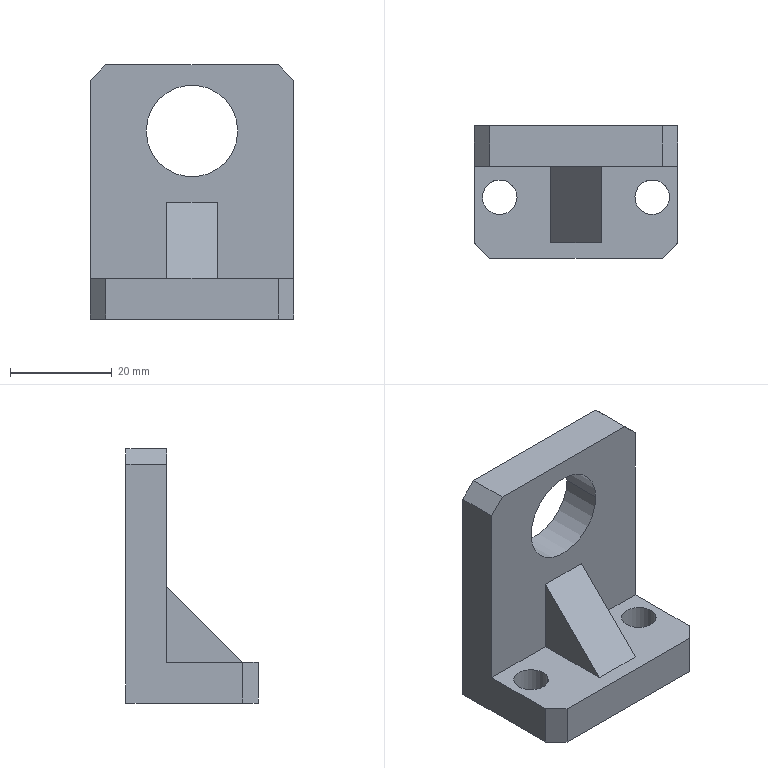Part | STEP file | 20315 | 1 solid | 21 faces | box 40 x 26 x 50 mm | volume 20124 mm3 | plane 15 | cylinder 6 | commonest cylinder face diameters 6.8 x4 18 x2
STEP:
#1=CARTESIAN_POINT('',(-17.984,13.63,0.));
#2=VERTEX_POINT('',#1);
#3=CARTESIAN_POINT('',(-17.984,13.63,8.));
#4=VERTEX_POINT('',#3);
#5=CARTESIAN_POINT('',(-17.984,13.63,24.155));
#6=DIRECTION('',(0.,0.,-1.));
#7=VECTOR('',#6,1.);
#8=LINE('',#5,#7);
#9=EDGE_CURVE('',#2,#4,#8,.F.);
#10=ORIENTED_EDGE('',*,*,#9,.F.);
#11=CARTESIAN_POINT('',(-12.016,10.37,0.));
#12=VERTEX_POINT('',#11);
#13=CARTESIAN_POINT('',(-15.,12.,0.));
#14=DIRECTION('',(0.,0.,-1.));
#15=AXIS2_PLACEMENT_3D('',#13,#14,$);
#16=CIRCLE('',#15,3.4);
#17=EDGE_CURVE('',#2,#12,#16,.T.);
#18=ORIENTED_EDGE('',*,*,#17,.T.);
#19=CARTESIAN_POINT('',(-12.016,10.37,8.));
#20=VERTEX_POINT('',#19);
#21=CARTESIAN_POINT('',(-12.016,10.37,24.155));
#22=DIRECTION('',(0.,0.,-1.));
#23=VECTOR('',#22,1.);
#24=LINE('',#21,#23);
#25=EDGE_CURVE('',#12,#20,#24,.F.);
#26=ORIENTED_EDGE('',*,*,#25,.T.);
#27=CARTESIAN_POINT('',(-15.,12.,8.));
#28=DIRECTION('',(0.,0.,-1.));
#29=AXIS2_PLACEMENT_3D('',#27,#28,$);
#30=CIRCLE('',#29,3.4);
#31=EDGE_CURVE('',#20,#4,#30,.F.);
#32=ORIENTED_EDGE('',*,*,#31,.T.);
#33=EDGE_LOOP('',(#10,#18,#26,#32));
#34=FACE_OUTER_BOUND('',#33,.T.);
#35=CARTESIAN_POINT('',(-15.,12.,7.9));
#36=DIRECTION('',(0.,0.,-1.));
#37=DIRECTION('',(0.8776,-0.4794,0.));
#38=AXIS2_PLACEMENT_3D('',#35,#36,#37);
#39=CYLINDRICAL_SURFACE('',#38,3.4);
#40=ADVANCED_FACE('',(#34),#39,.F.);
#41=ORIENTED_EDGE('',*,*,#25,.F.);
#42=CARTESIAN_POINT('',(-15.,12.,0.));
#43=DIRECTION('',(0.,0.,-1.));
#44=AXIS2_PLACEMENT_3D('',#42,#43,$);
#45=CIRCLE('',#44,3.4);
#46=EDGE_CURVE('',#12,#2,#45,.T.);
#47=ORIENTED_EDGE('',*,*,#46,.T.);
#48=ORIENTED_EDGE('',*,*,#9,.T.);
#49=CARTESIAN_POINT('',(-15.,12.,8.));
#50=DIRECTION('',(0.,0.,-1.));
#51=AXIS2_PLACEMENT_3D('',#49,#50,$);
#52=CIRCLE('',#51,3.4);
#53=EDGE_CURVE('',#4,#20,#52,.F.);
#54=ORIENTED_EDGE('',*,*,#53,.T.);
#55=EDGE_LOOP('',(#41,#47,#48,#54));
#56=FACE_OUTER_BOUND('',#55,.T.);
#57=ADVANCED_FACE('',(#56),#39,.F.);
#58=CARTESIAN_POINT('',(-5.,18.,8.));
#59=VERTEX_POINT('',#58);
#60=CARTESIAN_POINT('',(-5.,18.,23.));
#61=VERTEX_POINT('',#60);
#62=CARTESIAN_POINT('',(-5.,18.,15.5));
#63=DIRECTION('',(0.,0.,1.));
#64=VECTOR('',#63,1.);
#65=LINE('',#62,#64);
#66=EDGE_CURVE('',#59,#61,#65,.T.);
#67=ORIENTED_EDGE('',*,*,#66,.F.);
#68=CARTESIAN_POINT('',(-5.,3.,8.));
#69=VERTEX_POINT('',#68);
#70=CARTESIAN_POINT('',(-5.,10.5,8.));
#71=DIRECTION('',(0.,1.,0.));
#72=VECTOR('',#71,1.);
#73=LINE('',#70,#72);
#74=EDGE_CURVE('',#69,#59,#73,.T.);
#75=ORIENTED_EDGE('',*,*,#74,.F.);
#76=CARTESIAN_POINT('',(-5.,10.5,15.5));
#77=DIRECTION('',(0.,-0.7071,-0.7071));
#78=VECTOR('',#77,1.);
#79=LINE('',#76,#78);
#80=EDGE_CURVE('',#61,#69,#79,.T.);
#81=ORIENTED_EDGE('',*,*,#80,.F.);
#82=EDGE_LOOP('',(#67,#75,#81));
#83=FACE_OUTER_BOUND('',#82,.T.);
#84=CARTESIAN_POINT('',(-5.,0.,0.));
#85=DIRECTION('',(1.,0.,0.));
#86=DIRECTION('',(0.,1.,0.));
#87=AXIS2_PLACEMENT_3D('',#84,#85,#86);
#88=PLANE('',#87);
#89=ADVANCED_FACE('',(#83),#88,.F.);
#90=CARTESIAN_POINT('',(-20.,3.,8.));
#91=VERTEX_POINT('',#90);
#92=CARTESIAN_POINT('',(-20.,3.,0.));
#93=VERTEX_POINT('',#92);
#94=CARTESIAN_POINT('',(-20.,3.,4.));
#95=DIRECTION('',(0.,0.,-1.));
#96=VECTOR('',#95,1.);
#97=LINE('',#94,#96);
#98=EDGE_CURVE('',#91,#93,#97,.T.);
#99=ORIENTED_EDGE('',*,*,#98,.F.);
#100=CARTESIAN_POINT('',(-20.,18.,8.));
#101=VERTEX_POINT('',#100);
#102=CARTESIAN_POINT('',(-20.,10.5,8.));
#103=DIRECTION('',(0.,-1.,0.));
#104=VECTOR('',#103,1.);
#105=LINE('',#102,#104);
#106=EDGE_CURVE('',#101,#91,#105,.T.);
#107=ORIENTED_EDGE('',*,*,#106,.F.);
#108=CARTESIAN_POINT('',(-20.,18.,47.));
#109=VERTEX_POINT('',#108);
#110=CARTESIAN_POINT('',(-20.,18.,27.5));
#111=DIRECTION('',(0.,0.,-1.));
#112=VECTOR('',#111,1.);
#113=LINE('',#110,#112);
#114=EDGE_CURVE('',#109,#101,#113,.T.);
#115=ORIENTED_EDGE('',*,*,#114,.F.);
#116=CARTESIAN_POINT('',(-20.,26.,47.));
#117=VERTEX_POINT('',#116);
#118=CARTESIAN_POINT('',(-20.,22.,47.));
#119=DIRECTION('',(0.,1.,0.));
#120=VECTOR('',#119,1.);
#121=LINE('',#118,#120);
#122=EDGE_CURVE('',#117,#109,#121,.F.);
#123=ORIENTED_EDGE('',*,*,#122,.F.);
#124=CARTESIAN_POINT('',(-20.,26.,0.));
#125=VERTEX_POINT('',#124);
#126=CARTESIAN_POINT('',(-20.,26.,23.5));
#127=DIRECTION('',(0.,0.,1.));
#128=VECTOR('',#127,1.);
#129=LINE('',#126,#128);
#130=EDGE_CURVE('',#125,#117,#129,.T.);
#131=ORIENTED_EDGE('',*,*,#130,.F.);
#132=CARTESIAN_POINT('',(-20.,14.5,0.));
#133=DIRECTION('',(0.,1.,0.));
#134=VECTOR('',#133,1.);
#135=LINE('',#132,#134);
#136=EDGE_CURVE('',#93,#125,#135,.T.);
#137=ORIENTED_EDGE('',*,*,#136,.F.);
#138=EDGE_LOOP('',(#99,#107,#115,#123,#131,#137));
#139=FACE_OUTER_BOUND('',#138,.T.);
#140=CARTESIAN_POINT('',(-20.,0.,0.));
#141=DIRECTION('',(1.,0.,0.));
#142=DIRECTION('',(0.,1.,0.));
#143=AXIS2_PLACEMENT_3D('',#140,#141,#142);
#144=PLANE('',#143);
#145=ADVANCED_FACE('',(#139),#144,.F.);
#146=CARTESIAN_POINT('',(-17.,0.,8.));
#147=VERTEX_POINT('',#146);
#148=CARTESIAN_POINT('',(17.,0.,8.));
#149=VERTEX_POINT('',#148);
#150=CARTESIAN_POINT('',(0.,0.,8.));
#151=DIRECTION('',(1.,0.,0.));
#152=VECTOR('',#151,1.);
#153=LINE('',#150,#152);
#154=EDGE_CURVE('',#147,#149,#153,.T.);
#155=ORIENTED_EDGE('',*,*,#154,.F.);
#156=CARTESIAN_POINT('',(-17.,0.,0.));
#157=VERTEX_POINT('',#156);
#158=CARTESIAN_POINT('',(-17.,0.,4.));
#159=DIRECTION('',(0.,0.,-1.));
#160=VECTOR('',#159,1.);
#161=LINE('',#158,#160);
#162=EDGE_CURVE('',#147,#157,#161,.T.);
#163=ORIENTED_EDGE('',*,*,#162,.T.);
#164=CARTESIAN_POINT('',(17.,0.,0.));
#165=VERTEX_POINT('',#164);
#166=CARTESIAN_POINT('',(0.,0.,0.));
#167=DIRECTION('',(1.,0.,0.));
#168=VECTOR('',#167,1.);
#169=LINE('',#166,#168);
#170=EDGE_CURVE('',#157,#165,#169,.T.);
#171=ORIENTED_EDGE('',*,*,#170,.T.);
#172=CARTESIAN_POINT('',(17.,0.,4.));
#173=DIRECTION('',(0.,0.,-1.));
#174=VECTOR('',#173,1.);
#175=LINE('',#172,#174);
#176=EDGE_CURVE('',#149,#165,#175,.T.);
#177=ORIENTED_EDGE('',*,*,#176,.F.);
#178=EDGE_LOOP('',(#155,#163,#171,#177));
#179=FACE_OUTER_BOUND('',#178,.T.);
#180=CARTESIAN_POINT('',(0.,0.,8.));
#181=DIRECTION('',(0.,-1.,0.));
#182=DIRECTION('',(0.,0.,-1.));
#183=AXIS2_PLACEMENT_3D('',#180,#181,#182);
#184=PLANE('',#183);
#185=ADVANCED_FACE('',(#179),#184,.T.);
#186=CARTESIAN_POINT('',(-17.,18.,50.));
#187=VERTEX_POINT('',#186);
#188=CARTESIAN_POINT('',(17.,18.,50.));
#189=VERTEX_POINT('',#188);
#190=CARTESIAN_POINT('',(0.,18.,50.));
#191=DIRECTION('',(1.,0.,0.));
#192=VECTOR('',#191,1.);
#193=LINE('',#190,#192);
#194=EDGE_CURVE('',#187,#189,#193,.T.);
#195=ORIENTED_EDGE('',*,*,#194,.T.);
#196=CARTESIAN_POINT('',(17.,26.,50.));
#197=VERTEX_POINT('',#196);
#198=CARTESIAN_POINT('',(17.,22.,50.));
#199=DIRECTION('',(0.,1.,0.));
#200=VECTOR('',#199,1.);
#201=LINE('',#198,#200);
#202=EDGE_CURVE('',#197,#189,#201,.F.);
#203=ORIENTED_EDGE('',*,*,#202,.F.);
#204=CARTESIAN_POINT('',(-17.,26.,50.));
#205=VERTEX_POINT('',#204);
#206=CARTESIAN_POINT('',(0.,26.,50.));
#207=DIRECTION('',(1.,0.,0.));
#208=VECTOR('',#207,1.);
#209=LINE('',#206,#208);
#210=EDGE_CURVE('',#205,#197,#209,.T.);
#211=ORIENTED_EDGE('',*,*,#210,.F.);
#212=CARTESIAN_POINT('',(-17.,22.,50.));
#213=DIRECTION('',(0.,1.,0.));
#214=VECTOR('',#213,1.);
#215=LINE('',#212,#214);
#216=EDGE_CURVE('',#205,#187,#215,.F.);
#217=ORIENTED_EDGE('',*,*,#216,.T.);
#218=EDGE_LOOP('',(#195,#203,#211,#217));
#219=FACE_OUTER_BOUND('',#218,.T.);
#220=CARTESIAN_POINT('',(0.,26.,50.));
#221=DIRECTION('',(0.,0.,1.));
#222=DIRECTION('',(0.,-1.,0.));
#223=AXIS2_PLACEMENT_3D('',#220,#221,#222);
#224=PLANE('',#223);
#225=ADVANCED_FACE('',(#219),#224,.T.);
#226=CARTESIAN_POINT('',(20.,26.,47.));
#227=VERTEX_POINT('',#226);
#228=CARTESIAN_POINT('',(20.,18.,47.));
#229=VERTEX_POINT('',#228);
#230=CARTESIAN_POINT('',(20.,13.,47.));
#231=DIRECTION('',(0.,1.,0.));
#232=VECTOR('',#231,1.);
#233=LINE('',#230,#232);
#234=EDGE_CURVE('',#227,#229,#233,.F.);
#235=ORIENTED_EDGE('',*,*,#234,.F.);
#236=CARTESIAN_POINT('',(18.5,26.,48.5));
#237=DIRECTION('',(0.7071,0.,-0.7071));
#238=VECTOR('',#237,1.);
#239=LINE('',#236,#238);
#240=EDGE_CURVE('',#227,#197,#239,.F.);
#241=ORIENTED_EDGE('',*,*,#240,.T.);
#242=ORIENTED_EDGE('',*,*,#202,.T.);
#243=CARTESIAN_POINT('',(18.5,18.,48.5));
#244=DIRECTION('',(0.7071,0.,-0.7071));
#245=VECTOR('',#244,1.);
#246=LINE('',#243,#245);
#247=EDGE_CURVE('',#189,#229,#246,.T.);
#248=ORIENTED_EDGE('',*,*,#247,.T.);
#249=EDGE_LOOP('',(#235,#241,#242,#248));
#250=FACE_OUTER_BOUND('',#249,.T.);
#251=CARTESIAN_POINT('',(17.,-5.2,50.));
#252=DIRECTION('',(-0.7071,0.,-0.7071));
#253=DIRECTION('',(0.,1.,0.));
#254=AXIS2_PLACEMENT_3D('',#251,#252,#253);
#255=PLANE('',#254);
#256=ADVANCED_FACE('',(#250),#255,.F.);
#257=CARTESIAN_POINT('',(-18.5,18.,48.5));
#258=DIRECTION('',(-0.7071,0.,-0.7071));
#259=VECTOR('',#258,1.);
#260=LINE('',#257,#259);
#261=EDGE_CURVE('',#109,#187,#260,.F.);
#262=ORIENTED_EDGE('',*,*,#261,.T.);
#263=ORIENTED_EDGE('',*,*,#216,.F.);
#264=CARTESIAN_POINT('',(-18.5,26.,48.5));
#265=DIRECTION('',(-0.7071,0.,-0.7071));
#266=VECTOR('',#265,1.);
#267=LINE('',#264,#266);
#268=EDGE_CURVE('',#205,#117,#267,.T.);
#269=ORIENTED_EDGE('',*,*,#268,.T.);
#270=ORIENTED_EDGE('',*,*,#122,.T.);
#271=EDGE_LOOP('',(#262,#263,#269,#270));
#272=FACE_OUTER_BOUND('',#271,.T.);
#273=CARTESIAN_POINT('',(-17.,-5.2,50.));
#274=DIRECTION('',(-0.7071,0.,0.7071));
#275=DIRECTION('',(0.,1.,0.));
#276=AXIS2_PLACEMENT_3D('',#273,#274,#275);
#277=PLANE('',#276);
#278=ADVANCED_FACE('',(#272),#277,.T.);
#279=CARTESIAN_POINT('',(20.,3.,8.));
#280=VERTEX_POINT('',#279);
#281=CARTESIAN_POINT('',(20.,3.,0.));
#282=VERTEX_POINT('',#281);
#283=CARTESIAN_POINT('',(20.,3.,23.5));
#284=DIRECTION('',(0.,0.,-1.));
#285=VECTOR('',#284,1.);
#286=LINE('',#283,#285);
#287=EDGE_CURVE('',#280,#282,#286,.T.);
#288=ORIENTED_EDGE('',*,*,#287,.F.);
#289=CARTESIAN_POINT('',(18.5,1.5,8.));
#290=DIRECTION('',(-0.7071,-0.7071,0.));
#291=VECTOR('',#290,1.);
#292=LINE('',#289,#291);
#293=EDGE_CURVE('',#280,#149,#292,.T.);
#294=ORIENTED_EDGE('',*,*,#293,.T.);
#295=ORIENTED_EDGE('',*,*,#176,.T.);
#296=CARTESIAN_POINT('',(18.5,1.5,0.));
#297=DIRECTION('',(-0.7071,-0.7071,0.));
#298=VECTOR('',#297,1.);
#299=LINE('',#296,#298);
#300=EDGE_CURVE('',#165,#282,#299,.F.);
#301=ORIENTED_EDGE('',*,*,#300,.T.);
#302=EDGE_LOOP('',(#288,#294,#295,#301));
#303=FACE_OUTER_BOUND('',#302,.T.);
#304=CARTESIAN_POINT('',(20.,3.,56.4));
#305=DIRECTION('',(-0.7071,0.7071,0.));
#306=DIRECTION('',(0.,0.,-1.));
#307=AXIS2_PLACEMENT_3D('',#304,#305,#306);
#308=PLANE('',#307);
#309=ADVANCED_FACE('',(#303),#308,.F.);
#310=CARTESIAN_POINT('',(-18.5,1.5,0.));
#311=DIRECTION('',(0.7071,-0.7071,0.));
#312=VECTOR('',#311,1.);
#313=LINE('',#310,#312);
#314=EDGE_CURVE('',#93,#157,#313,.T.);
#315=ORIENTED_EDGE('',*,*,#314,.T.);
#316=ORIENTED_EDGE('',*,*,#162,.F.);
#317=CARTESIAN_POINT('',(-18.5,1.5,8.));
#318=DIRECTION('',(0.7071,-0.7071,0.));
#319=VECTOR('',#318,1.);
#320=LINE('',#317,#319);
#321=EDGE_CURVE('',#147,#91,#320,.F.);
#322=ORIENTED_EDGE('',*,*,#321,.T.);
#323=ORIENTED_EDGE('',*,*,#98,.T.);
#324=EDGE_LOOP('',(#315,#316,#322,#323));
#325=FACE_OUTER_BOUND('',#324,.T.);
#326=CARTESIAN_POINT('',(-20.,3.,56.4));
#327=DIRECTION('',(-0.7071,-0.7071,0.));
#328=DIRECTION('',(0.,0.,-1.));
#329=AXIS2_PLACEMENT_3D('',#326,#327,#328);
#330=PLANE('',#329);
#331=ADVANCED_FACE('',(#325),#330,.T.);
#332=CARTESIAN_POINT('',(5.,18.,23.));
#333=VERTEX_POINT('',#332);
#334=CARTESIAN_POINT('',(0.,18.,23.));
#335=DIRECTION('',(1.,0.,0.));
#336=VECTOR('',#335,1.);
#337=LINE('',#334,#336);
#338=EDGE_CURVE('',#61,#333,#337,.T.);
#339=ORIENTED_EDGE('',*,*,#338,.F.);
#340=ORIENTED_EDGE('',*,*,#80,.T.);
#341=CARTESIAN_POINT('',(5.,3.,8.));
#342=VERTEX_POINT('',#341);
#343=CARTESIAN_POINT('',(0.,3.,8.));
#344=DIRECTION('',(1.,0.,0.));
#345=VECTOR('',#344,1.);
#346=LINE('',#343,#345);
#347=EDGE_CURVE('',#69,#342,#346,.T.);
#348=ORIENTED_EDGE('',*,*,#347,.T.);
#349=CARTESIAN_POINT('',(5.,10.5,15.5));
#350=DIRECTION('',(0.,-0.7071,-0.7071));
#351=VECTOR('',#350,1.);
#352=LINE('',#349,#351);
#353=EDGE_CURVE('',#333,#342,#352,.T.);
#354=ORIENTED_EDGE('',*,*,#353,.F.);
#355=EDGE_LOOP('',(#339,#340,#348,#354));
#356=FACE_OUTER_BOUND('',#355,.T.);
#357=CARTESIAN_POINT('',(0.,18.,23.));
#358=DIRECTION('',(0.,-0.7071,0.7071));
#359=DIRECTION('',(0.,-0.7071,-0.7071));
#360=AXIS2_PLACEMENT_3D('',#357,#358,#359);
#361=PLANE('',#360);
#362=ADVANCED_FACE('',(#356),#361,.T.);
#363=ORIENTED_EDGE('',*,*,#353,.T.);
#364=CARTESIAN_POINT('',(5.,18.,8.));
#365=VERTEX_POINT('',#364);
#366=CARTESIAN_POINT('',(5.,10.5,8.));
#367=DIRECTION('',(0.,1.,0.));
#368=VECTOR('',#367,1.);
#369=LINE('',#366,#368);
#370=EDGE_CURVE('',#342,#365,#369,.T.);
#371=ORIENTED_EDGE('',*,*,#370,.T.);
#372=CARTESIAN_POINT('',(5.,18.,15.5));
#373=DIRECTION('',(0.,0.,1.));
#374=VECTOR('',#373,1.);
#375=LINE('',#372,#374);
#376=EDGE_CURVE('',#365,#333,#375,.T.);
#377=ORIENTED_EDGE('',*,*,#376,.T.);
#378=EDGE_LOOP('',(#363,#371,#377));
#379=FACE_OUTER_BOUND('',#378,.T.);
#380=CARTESIAN_POINT('',(5.,0.,0.));
#381=DIRECTION('',(1.,0.,0.));
#382=DIRECTION('',(0.,1.,0.));
#383=AXIS2_PLACEMENT_3D('',#380,#381,#382);
#384=PLANE('',#383);
#385=ADVANCED_FACE('',(#379),#384,.T.);
#386=CARTESIAN_POINT('',(20.,26.,0.));
#387=VERTEX_POINT('',#386);
#388=CARTESIAN_POINT('',(20.,14.5,0.));
#389=DIRECTION('',(0.,1.,0.));
#390=VECTOR('',#389,1.);
#391=LINE('',#388,#390);
#392=EDGE_CURVE('',#282,#387,#391,.T.);
#393=ORIENTED_EDGE('',*,*,#392,.T.);
#394=CARTESIAN_POINT('',(20.,26.,23.5));
#395=DIRECTION('',(0.,0.,1.));
#396=VECTOR('',#395,1.);
#397=LINE('',#394,#396);
#398=EDGE_CURVE('',#387,#227,#397,.T.);
#399=ORIENTED_EDGE('',*,*,#398,.T.);
#400=ORIENTED_EDGE('',*,*,#234,.T.);
#401=CARTESIAN_POINT('',(20.,18.,8.));
#402=VERTEX_POINT('',#401);
#403=CARTESIAN_POINT('',(20.,18.,27.5));
#404=DIRECTION('',(0.,0.,-1.));
#405=VECTOR('',#404,1.);
#406=LINE('',#403,#405);
#407=EDGE_CURVE('',#229,#402,#406,.T.);
#408=ORIENTED_EDGE('',*,*,#407,.T.);
#409=CARTESIAN_POINT('',(20.,10.5,8.));
#410=DIRECTION('',(0.,-1.,0.));
#411=VECTOR('',#410,1.);
#412=LINE('',#409,#411);
#413=EDGE_CURVE('',#402,#280,#412,.T.);
#414=ORIENTED_EDGE('',*,*,#413,.T.);
#415=ORIENTED_EDGE('',*,*,#287,.T.);
#416=EDGE_LOOP('',(#393,#399,#400,#408,#414,#415));
#417=FACE_OUTER_BOUND('',#416,.T.);
#418=CARTESIAN_POINT('',(20.,0.,0.));
#419=DIRECTION('',(1.,0.,0.));
#420=DIRECTION('',(0.,1.,0.));
#421=AXIS2_PLACEMENT_3D('',#418,#419,#420);
#422=PLANE('',#421);
#423=ADVANCED_FACE('',(#417),#422,.T.);
#424=ORIENTED_EDGE('',*,*,#170,.F.);
#425=ORIENTED_EDGE('',*,*,#314,.F.);
#426=ORIENTED_EDGE('',*,*,#136,.T.);
#427=CARTESIAN_POINT('',(0.,26.,0.));
#428=DIRECTION('',(1.,0.,0.));
#429=VECTOR('',#428,1.);
#430=LINE('',#427,#429);
#431=EDGE_CURVE('',#125,#387,#430,.T.);
#432=ORIENTED_EDGE('',*,*,#431,.T.);
#433=ORIENTED_EDGE('',*,*,#392,.F.);
#434=ORIENTED_EDGE('',*,*,#300,.F.);
#435=EDGE_LOOP('',(#424,#425,#426,#432,#433,#434));
#436=FACE_OUTER_BOUND('',#435,.T.);
#437=CARTESIAN_POINT('',(12.016,13.63,0.));
#438=VERTEX_POINT('',#437);
#439=CARTESIAN_POINT('',(17.984,10.37,0.));
#440=VERTEX_POINT('',#439);
#441=CARTESIAN_POINT('',(15.,12.,0.));
#442=DIRECTION('',(0.,0.,-1.));
#443=AXIS2_PLACEMENT_3D('',#441,#442,$);
#444=CIRCLE('',#443,3.4);
#445=EDGE_CURVE('',#438,#440,#444,.T.);
#446=ORIENTED_EDGE('',*,*,#445,.F.);
#447=CARTESIAN_POINT('',(15.,12.,0.));
#448=DIRECTION('',(0.,0.,-1.));
#449=AXIS2_PLACEMENT_3D('',#447,#448,$);
#450=CIRCLE('',#449,3.4);
#451=EDGE_CURVE('',#440,#438,#450,.T.);
#452=ORIENTED_EDGE('',*,*,#451,.F.);
#453=EDGE_LOOP('',(#446,#452));
#454=FACE_BOUND('',#453,.T.);
#455=ORIENTED_EDGE('',*,*,#46,.F.);
#456=ORIENTED_EDGE('',*,*,#17,.F.);
#457=EDGE_LOOP('',(#455,#456));
#458=FACE_BOUND('',#457,.T.);
#459=CARTESIAN_POINT('',(0.,0.,0.));
#460=DIRECTION('',(0.,0.,-1.));
#461=DIRECTION('',(0.,1.,0.));
#462=AXIS2_PLACEMENT_3D('',#459,#460,#461);
#463=PLANE('',#462);
#464=ADVANCED_FACE('',(#436,#454,#458),#463,.T.);
#465=ORIENTED_EDGE('',*,*,#413,.F.);
#466=CARTESIAN_POINT('',(12.5,18.,8.));
#467=DIRECTION('',(1.,0.,0.));
#468=VECTOR('',#467,1.);
#469=LINE('',#466,#468);
#470=EDGE_CURVE('',#365,#402,#469,.T.);
#471=ORIENTED_EDGE('',*,*,#470,.F.);
#472=ORIENTED_EDGE('',*,*,#370,.F.);
#473=ORIENTED_EDGE('',*,*,#347,.F.);
#474=ORIENTED_EDGE('',*,*,#74,.T.);
#475=CARTESIAN_POINT('',(-12.5,18.,8.));
#476=DIRECTION('',(1.,0.,0.));
#477=VECTOR('',#476,1.);
#478=LINE('',#475,#477);
#479=EDGE_CURVE('',#101,#59,#478,.T.);
#480=ORIENTED_EDGE('',*,*,#479,.F.);
#481=ORIENTED_EDGE('',*,*,#106,.T.);
#482=ORIENTED_EDGE('',*,*,#321,.F.);
#483=ORIENTED_EDGE('',*,*,#154,.T.);
#484=ORIENTED_EDGE('',*,*,#293,.F.);
#485=EDGE_LOOP('',(#465,#471,#472,#473,#474,#480,#481,#482,#483,#484));
#486=FACE_OUTER_BOUND('',#485,.T.);
#487=CARTESIAN_POINT('',(17.984,10.37,8.));
#488=VERTEX_POINT('',#487);
#489=CARTESIAN_POINT('',(12.016,13.63,8.));
#490=VERTEX_POINT('',#489);
#491=CARTESIAN_POINT('',(15.,12.,8.));
#492=DIRECTION('',(0.,0.,1.));
#493=AXIS2_PLACEMENT_3D('',#491,#492,$);
#494=CIRCLE('',#493,3.4);
#495=EDGE_CURVE('',#488,#490,#494,.T.);
#496=ORIENTED_EDGE('',*,*,#495,.F.);
#497=CARTESIAN_POINT('',(15.,12.,8.));
#498=DIRECTION('',(0.,0.,1.));
#499=AXIS2_PLACEMENT_3D('',#497,#498,$);
#500=CIRCLE('',#499,3.4);
#501=EDGE_CURVE('',#490,#488,#500,.T.);
#502=ORIENTED_EDGE('',*,*,#501,.F.);
#503=EDGE_LOOP('',(#496,#502));
#504=FACE_BOUND('',#503,.T.);
#505=ORIENTED_EDGE('',*,*,#53,.F.);
#506=ORIENTED_EDGE('',*,*,#31,.F.);
#507=EDGE_LOOP('',(#505,#506));
#508=FACE_BOUND('',#507,.T.);
#509=CARTESIAN_POINT('',(0.,18.,8.));
#510=DIRECTION('',(0.,0.,1.));
#511=DIRECTION('',(0.,-1.,0.));
#512=AXIS2_PLACEMENT_3D('',#509,#510,#511);
#513=PLANE('',#512);
#514=ADVANCED_FACE('',(#486,#504,#508),#513,.T.);
#515=CARTESIAN_POINT('',(12.016,13.63,24.155));
#516=DIRECTION('',(0.,0.,-1.));
#517=VECTOR('',#516,1.);
#518=LINE('',#515,#517);
#519=EDGE_CURVE('',#438,#490,#518,.F.);
#520=ORIENTED_EDGE('',*,*,#519,.F.);
#521=ORIENTED_EDGE('',*,*,#445,.T.);
#522=CARTESIAN_POINT('',(17.984,10.37,24.155));
#523=DIRECTION('',(0.,0.,-1.));
#524=VECTOR('',#523,1.);
#525=LINE('',#522,#524);
#526=EDGE_CURVE('',#440,#488,#525,.F.);
#527=ORIENTED_EDGE('',*,*,#526,.T.);
#528=ORIENTED_EDGE('',*,*,#495,.T.);
#529=EDGE_LOOP('',(#520,#521,#527,#528));
#530=FACE_OUTER_BOUND('',#529,.T.);
#531=CARTESIAN_POINT('',(15.,12.,7.9));
#532=DIRECTION('',(0.,0.,-1.));
#533=DIRECTION('',(0.8776,-0.4794,0.));
#534=AXIS2_PLACEMENT_3D('',#531,#532,#533);
#535=CYLINDRICAL_SURFACE('',#534,3.4);
#536=ADVANCED_FACE('',(#530),#535,.F.);
#537=ORIENTED_EDGE('',*,*,#526,.F.);
#538=ORIENTED_EDGE('',*,*,#451,.T.);
#539=ORIENTED_EDGE('',*,*,#519,.T.);
#540=ORIENTED_EDGE('',*,*,#501,.T.);
#541=EDGE_LOOP('',(#537,#538,#539,#540));
#542=FACE_OUTER_BOUND('',#541,.T.);
#543=ADVANCED_FACE('',(#542),#535,.F.);
#544=ORIENTED_EDGE('',*,*,#470,.T.);
#545=ORIENTED_EDGE('',*,*,#407,.F.);
#546=ORIENTED_EDGE('',*,*,#247,.F.);
#547=ORIENTED_EDGE('',*,*,#194,.F.);
#548=ORIENTED_EDGE('',*,*,#261,.F.);
#549=ORIENTED_EDGE('',*,*,#114,.T.);
#550=ORIENTED_EDGE('',*,*,#479,.T.);
#551=ORIENTED_EDGE('',*,*,#66,.T.);
#552=ORIENTED_EDGE('',*,*,#338,.T.);
#553=ORIENTED_EDGE('',*,*,#376,.F.);
#554=EDGE_LOOP('',(#544,#545,#546,#547,#548,#549,#550,#551,#552,#553));
#555=FACE_OUTER_BOUND('',#554,.T.);
#556=CARTESIAN_POINT('',(9.,18.,37.));
#557=VERTEX_POINT('',#556);
#558=CARTESIAN_POINT('',(-9.,18.,37.));
#559=VERTEX_POINT('',#558);
#560=CARTESIAN_POINT('',(0.,18.,37.));
#561=DIRECTION('',(0.,-1.,0.));
#562=AXIS2_PLACEMENT_3D('',#560,#561,$);
#563=CIRCLE('',#562,9.);
#564=EDGE_CURVE('',#557,#559,#563,.T.);
#565=ORIENTED_EDGE('',*,*,#564,.F.);
#566=CARTESIAN_POINT('',(0.,18.,37.));
#567=DIRECTION('',(0.,-1.,0.));
#568=AXIS2_PLACEMENT_3D('',#566,#567,$);
#569=CIRCLE('',#568,9.);
#570=EDGE_CURVE('',#559,#557,#569,.T.);
#571=ORIENTED_EDGE('',*,*,#570,.F.);
#572=EDGE_LOOP('',(#565,#571));
#573=FACE_BOUND('',#572,.T.);
#574=CARTESIAN_POINT('',(0.,18.,50.));
#575=DIRECTION('',(0.,-1.,0.));
#576=DIRECTION('',(0.,0.,-1.));
#577=AXIS2_PLACEMENT_3D('',#574,#575,#576);
#578=PLANE('',#577);
#579=ADVANCED_FACE('',(#555,#573),#578,.T.);
#580=ORIENTED_EDGE('',*,*,#210,.T.);
#581=ORIENTED_EDGE('',*,*,#240,.F.);
#582=ORIENTED_EDGE('',*,*,#398,.F.);
#583=ORIENTED_EDGE('',*,*,#431,.F.);
#584=ORIENTED_EDGE('',*,*,#130,.T.);
#585=ORIENTED_EDGE('',*,*,#268,.F.);
#586=EDGE_LOOP('',(#580,#581,#582,#583,#584,#585));
#587=FACE_OUTER_BOUND('',#586,.T.);
#588=CARTESIAN_POINT('',(-9.,26.,37.));
#589=VERTEX_POINT('',#588);
#590=CARTESIAN_POINT('',(9.,26.,37.));
#591=VERTEX_POINT('',#590);
#592=CARTESIAN_POINT('',(0.,26.,37.));
#593=DIRECTION('',(0.,1.,0.));
#594=AXIS2_PLACEMENT_3D('',#592,#593,$);
#595=CIRCLE('',#594,9.);
#596=EDGE_CURVE('',#589,#591,#595,.T.);
#597=ORIENTED_EDGE('',*,*,#596,.F.);
#598=CARTESIAN_POINT('',(0.,26.,37.));
#599=DIRECTION('',(0.,1.,0.));
#600=AXIS2_PLACEMENT_3D('',#598,#599,$);
#601=CIRCLE('',#600,9.);
#602=EDGE_CURVE('',#591,#589,#601,.T.);
#603=ORIENTED_EDGE('',*,*,#602,.F.);
#604=EDGE_LOOP('',(#597,#603));
#605=FACE_BOUND('',#604,.T.);
#606=CARTESIAN_POINT('',(0.,26.,0.));
#607=DIRECTION('',(0.,1.,0.));
#608=DIRECTION('',(0.,0.,1.));
#609=AXIS2_PLACEMENT_3D('',#606,#607,#608);
#610=PLANE('',#609);
#611=ADVANCED_FACE('',(#587,#605),#610,.T.);
#612=CARTESIAN_POINT('',(9.,21.,37.));
#613=DIRECTION('',(0.,-1.,0.));
#614=VECTOR('',#613,1.);
#615=LINE('',#612,#614);
#616=EDGE_CURVE('',#557,#591,#615,.F.);
#617=ORIENTED_EDGE('',*,*,#616,.T.);
#618=ORIENTED_EDGE('',*,*,#602,.T.);
#619=CARTESIAN_POINT('',(-9.,21.,37.));
#620=DIRECTION('',(0.,-1.,0.));
#621=VECTOR('',#620,1.);
#622=LINE('',#619,#621);
#623=EDGE_CURVE('',#559,#589,#622,.F.);
#624=ORIENTED_EDGE('',*,*,#623,.F.);
#625=ORIENTED_EDGE('',*,*,#570,.T.);
#626=EDGE_LOOP('',(#617,#618,#624,#625));
#627=FACE_OUTER_BOUND('',#626,.T.);
#628=CARTESIAN_POINT('',(0.,21.,37.));
#629=DIRECTION('',(0.,-1.,0.));
#630=DIRECTION('',(1.,0.,0.));
#631=AXIS2_PLACEMENT_3D('',#628,#629,#630);
#632=CYLINDRICAL_SURFACE('',#631,9.);
#633=ADVANCED_FACE('',(#627),#632,.F.);
#634=ORIENTED_EDGE('',*,*,#623,.T.);
#635=ORIENTED_EDGE('',*,*,#596,.T.);
#636=ORIENTED_EDGE('',*,*,#616,.F.);
#637=ORIENTED_EDGE('',*,*,#564,.T.);
#638=EDGE_LOOP('',(#634,#635,#636,#637));
#639=FACE_OUTER_BOUND('',#638,.T.);
#640=ADVANCED_FACE('',(#639),#632,.F.);
#641=CLOSED_SHELL('',(#40,#57,#89,#145,#185,#225,#256,#278,#309,#331,#362,#385,#423,#464,#514,#536,#543,#579,#611,#633,#640));
#642=MANIFOLD_SOLID_BREP('',#641);
#643=(LENGTH_UNIT()NAMED_UNIT(*)SI_UNIT(.MILLI.,.METRE.));
#644=UNCERTAINTY_MEASURE_WITH_UNIT(LENGTH_MEASURE(0.005),#643,'','');
#645=(NAMED_UNIT(*)PLANE_ANGLE_UNIT()SI_UNIT($,.RADIAN.));
#646=(NAMED_UNIT(*)SI_UNIT($,.STERADIAN.)SOLID_ANGLE_UNIT());
#647=(GEOMETRIC_REPRESENTATION_CONTEXT(3)GLOBAL_UNCERTAINTY_ASSIGNED_CONTEXT((#644))GLOBAL_UNIT_ASSIGNED_CONTEXT((#643,#645,#646))REPRESENTATION_CONTEXT('',''));
#648=ADVANCED_BREP_SHAPE_REPRESENTATION('',(#642),#647);